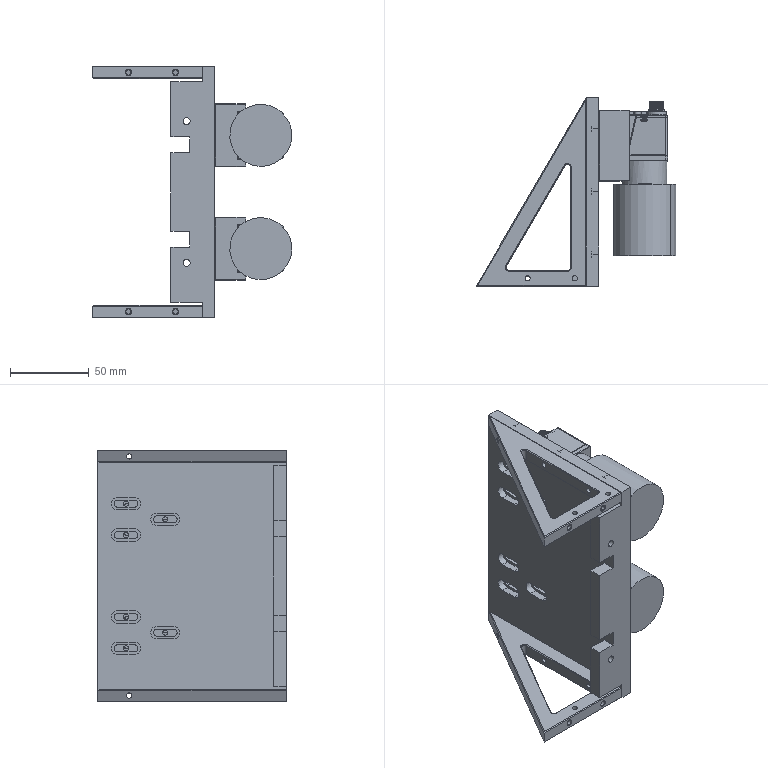Part | SolidWorks | 7 solids | 3224 faces | volume 422157 mm3 | plane 1742 | cylinder 896 | spline 340 | cone 240 | torus 6 | commonest cylinder face diameters 0.4 x168 1.4 x78 8.5 x42 2 x40 3.3 x40 8 x38